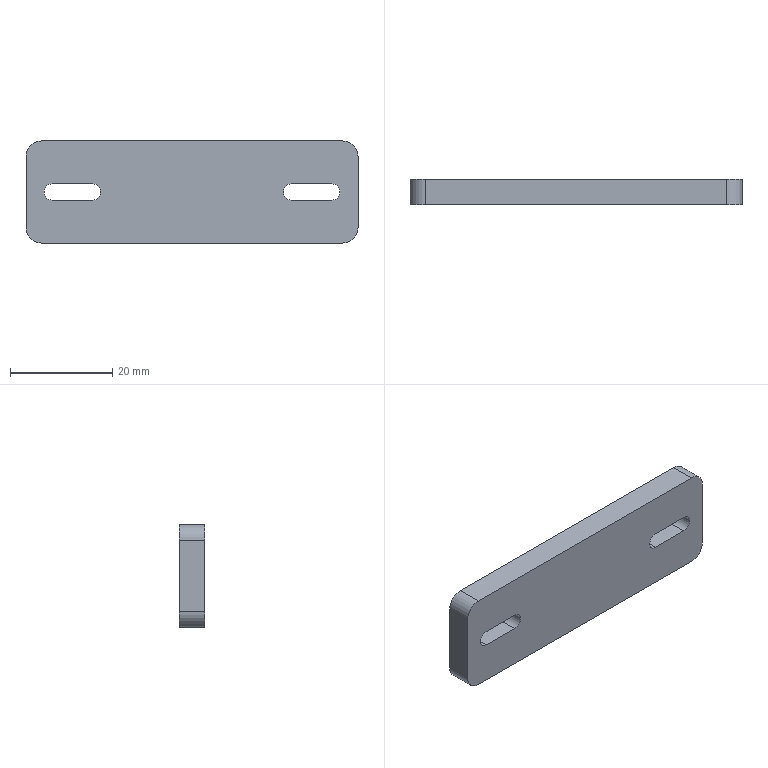Part | SolidWorks | features BaseBody 1 | 1 solid | 18 faces | box 65 x 5 x 20 mm | volume 6129 mm3 | plane 10 | cylinder 8 | commonest cylinder face diameters 3.2 x4 6 x4
STEP:
#1=CARTESIAN_POINT('',(32.5,5.,7.));
#2=VERTEX_POINT('',#1);
#3=CARTESIAN_POINT('',(32.5,5.,-7.));
#4=VERTEX_POINT('',#3);
#5=CARTESIAN_POINT('',(32.5,5.,0.));
#6=DIRECTION('',(0.,0.,-1.));
#7=VECTOR('',#6,1000.);
#8=LINE('',#5,#7);
#9=EDGE_CURVE('',#2,#4,#8,.T.);
#10=ORIENTED_EDGE('',*,*,#9,.T.);
#11=CARTESIAN_POINT('',(29.5,5.,-10.));
#12=VERTEX_POINT('',#11);
#13=CARTESIAN_POINT('',(29.5,5.,-7.));
#14=DIRECTION('',(0.,1.,0.));
#15=DIRECTION('',(0.,0.,-1.));
#16=AXIS2_PLACEMENT_3D('',#13,#14,#15);
#17=CIRCLE('',#16,3.);
#18=EDGE_CURVE('',#4,#12,#17,.T.);
#19=ORIENTED_EDGE('',*,*,#18,.T.);
#20=CARTESIAN_POINT('',(-29.5,5.,-10.));
#21=VERTEX_POINT('',#20);
#22=CARTESIAN_POINT('',(0.,5.,-10.));
#23=DIRECTION('',(-1.,0.,0.));
#24=VECTOR('',#23,1000.);
#25=LINE('',#22,#24);
#26=EDGE_CURVE('',#12,#21,#25,.T.);
#27=ORIENTED_EDGE('',*,*,#26,.T.);
#28=CARTESIAN_POINT('',(-32.5,5.,-7.));
#29=VERTEX_POINT('',#28);
#30=CARTESIAN_POINT('',(-29.5,5.,-7.));
#31=DIRECTION('',(0.,1.,0.));
#32=DIRECTION('',(0.,0.,-1.));
#33=AXIS2_PLACEMENT_3D('',#30,#31,#32);
#34=CIRCLE('',#33,3.);
#35=EDGE_CURVE('',#21,#29,#34,.T.);
#36=ORIENTED_EDGE('',*,*,#35,.T.);
#37=CARTESIAN_POINT('',(-32.5,5.,7.));
#38=VERTEX_POINT('',#37);
#39=CARTESIAN_POINT('',(-32.5,5.,0.));
#40=DIRECTION('',(0.,0.,1.));
#41=VECTOR('',#40,1000.);
#42=LINE('',#39,#41);
#43=EDGE_CURVE('',#29,#38,#42,.T.);
#44=ORIENTED_EDGE('',*,*,#43,.T.);
#45=CARTESIAN_POINT('',(-29.5,5.,10.));
#46=VERTEX_POINT('',#45);
#47=CARTESIAN_POINT('',(-29.5,5.,7.));
#48=DIRECTION('',(0.,1.,0.));
#49=DIRECTION('',(0.,0.,-1.));
#50=AXIS2_PLACEMENT_3D('',#47,#48,#49);
#51=CIRCLE('',#50,3.);
#52=EDGE_CURVE('',#38,#46,#51,.T.);
#53=ORIENTED_EDGE('',*,*,#52,.T.);
#54=CARTESIAN_POINT('',(29.5,5.,10.));
#55=VERTEX_POINT('',#54);
#56=CARTESIAN_POINT('',(0.,5.,10.));
#57=DIRECTION('',(1.,0.,0.));
#58=VECTOR('',#57,1000.);
#59=LINE('',#56,#58);
#60=EDGE_CURVE('',#46,#55,#59,.T.);
#61=ORIENTED_EDGE('',*,*,#60,.T.);
#62=CARTESIAN_POINT('',(29.5,5.,7.));
#63=DIRECTION('',(0.,1.,0.));
#64=DIRECTION('',(0.,0.,-1.));
#65=AXIS2_PLACEMENT_3D('',#62,#63,#64);
#66=CIRCLE('',#65,3.);
#67=EDGE_CURVE('',#55,#2,#66,.T.);
#68=ORIENTED_EDGE('',*,*,#67,.T.);
#69=EDGE_LOOP('',(#10,#19,#27,#36,#44,#53,#61,#68));
#70=FACE_OUTER_BOUND('',#69,.T.);
#71=CARTESIAN_POINT('',(19.5,5.,1.6));
#72=VERTEX_POINT('',#71);
#73=CARTESIAN_POINT('',(19.5,5.,-1.6));
#74=VERTEX_POINT('',#73);
#75=CARTESIAN_POINT('',(19.5,5.,0.));
#76=DIRECTION('',(0.,-1.,0.));
#77=DIRECTION('',(0.,0.,1.));
#78=AXIS2_PLACEMENT_3D('',#75,#76,#77);
#79=CIRCLE('',#78,1.6);
#80=EDGE_CURVE('',#72,#74,#79,.T.);
#81=ORIENTED_EDGE('',*,*,#80,.T.);
#82=CARTESIAN_POINT('',(27.375,5.,-1.6));
#83=VERTEX_POINT('',#82);
#84=CARTESIAN_POINT('',(0.,5.,-1.6));
#85=DIRECTION('',(1.,0.,0.));
#86=VECTOR('',#85,1000.);
#87=LINE('',#84,#86);
#88=EDGE_CURVE('',#74,#83,#87,.T.);
#89=ORIENTED_EDGE('',*,*,#88,.T.);
#90=CARTESIAN_POINT('',(27.375,5.,1.6));
#91=VERTEX_POINT('',#90);
#92=CARTESIAN_POINT('',(27.375,5.,0.));
#93=DIRECTION('',(0.,-1.,0.));
#94=DIRECTION('',(0.,0.,1.));
#95=AXIS2_PLACEMENT_3D('',#92,#93,#94);
#96=CIRCLE('',#95,1.6);
#97=EDGE_CURVE('',#83,#91,#96,.T.);
#98=ORIENTED_EDGE('',*,*,#97,.T.);
#99=CARTESIAN_POINT('',(0.,5.,1.6));
#100=DIRECTION('',(-1.,0.,0.));
#101=VECTOR('',#100,1000.);
#102=LINE('',#99,#101);
#103=EDGE_CURVE('',#91,#72,#102,.T.);
#104=ORIENTED_EDGE('',*,*,#103,.T.);
#105=EDGE_LOOP('',(#81,#89,#98,#104));
#106=FACE_BOUND('',#105,.T.);
#107=CARTESIAN_POINT('',(-19.5,5.,-1.6));
#108=VERTEX_POINT('',#107);
#109=CARTESIAN_POINT('',(-19.5,5.,1.6));
#110=VERTEX_POINT('',#109);
#111=CARTESIAN_POINT('',(-19.5,5.,0.));
#112=DIRECTION('',(0.,-1.,0.));
#113=DIRECTION('',(0.,0.,1.));
#114=AXIS2_PLACEMENT_3D('',#111,#112,#113);
#115=CIRCLE('',#114,1.6);
#116=EDGE_CURVE('',#108,#110,#115,.T.);
#117=ORIENTED_EDGE('',*,*,#116,.T.);
#118=CARTESIAN_POINT('',(-27.375,5.,1.6));
#119=VERTEX_POINT('',#118);
#120=CARTESIAN_POINT('',(0.,5.,1.6));
#121=DIRECTION('',(-1.,0.,0.));
#122=VECTOR('',#121,1000.);
#123=LINE('',#120,#122);
#124=EDGE_CURVE('',#110,#119,#123,.T.);
#125=ORIENTED_EDGE('',*,*,#124,.T.);
#126=CARTESIAN_POINT('',(-27.375,5.,-1.6));
#127=VERTEX_POINT('',#126);
#128=CARTESIAN_POINT('',(-27.375,5.,0.));
#129=DIRECTION('',(0.,-1.,0.));
#130=DIRECTION('',(0.,0.,1.));
#131=AXIS2_PLACEMENT_3D('',#128,#129,#130);
#132=CIRCLE('',#131,1.6);
#133=EDGE_CURVE('',#119,#127,#132,.T.);
#134=ORIENTED_EDGE('',*,*,#133,.T.);
#135=CARTESIAN_POINT('',(0.,5.,-1.6));
#136=DIRECTION('',(1.,0.,0.));
#137=VECTOR('',#136,1000.);
#138=LINE('',#135,#137);
#139=EDGE_CURVE('',#127,#108,#138,.T.);
#140=ORIENTED_EDGE('',*,*,#139,.T.);
#141=EDGE_LOOP('',(#117,#125,#134,#140));
#142=FACE_BOUND('',#141,.T.);
#143=CARTESIAN_POINT('',(0.,5.,0.));
#144=DIRECTION('',(0.,1.,0.));
#145=DIRECTION('',(0.,0.,1.));
#146=AXIS2_PLACEMENT_3D('',#143,#144,#145);
#147=PLANE('',#146);
#148=ADVANCED_FACE('',(#70,#106,#142),#147,.T.);
#149=CARTESIAN_POINT('',(32.5,0.,-7.));
#150=VERTEX_POINT('',#149);
#151=CARTESIAN_POINT('',(29.5,0.,-10.));
#152=VERTEX_POINT('',#151);
#153=CARTESIAN_POINT('',(29.5,0.,-7.));
#154=DIRECTION('',(0.,1.,0.));
#155=DIRECTION('',(0.,0.,-1.));
#156=AXIS2_PLACEMENT_3D('',#153,#154,#155);
#157=CIRCLE('',#156,3.);
#158=EDGE_CURVE('',#150,#152,#157,.T.);
#159=ORIENTED_EDGE('',*,*,#158,.T.);
#160=CARTESIAN_POINT('',(29.5,5.,-10.));
#161=DIRECTION('',(0.,1.,0.));
#162=VECTOR('',#161,1000.);
#163=LINE('',#160,#162);
#164=EDGE_CURVE('',#152,#12,#163,.T.);
#165=ORIENTED_EDGE('',*,*,#164,.T.);
#166=ORIENTED_EDGE('',*,*,#18,.F.);
#167=CARTESIAN_POINT('',(32.5,5.,-7.));
#168=DIRECTION('',(0.,-1.,0.));
#169=VECTOR('',#168,1000.);
#170=LINE('',#167,#169);
#171=EDGE_CURVE('',#4,#150,#170,.T.);
#172=ORIENTED_EDGE('',*,*,#171,.T.);
#173=EDGE_LOOP('',(#159,#165,#166,#172));
#174=FACE_OUTER_BOUND('',#173,.T.);
#175=CARTESIAN_POINT('',(29.5,5.,-7.));
#176=DIRECTION('',(0.,-1.,0.));
#177=DIRECTION('',(0.,0.,-1.));
#178=AXIS2_PLACEMENT_3D('',#175,#176,#177);
#179=CYLINDRICAL_SURFACE('',#178,3.);
#180=ADVANCED_FACE('',(#174),#179,.T.);
#181=ORIENTED_EDGE('',*,*,#171,.F.);
#182=ORIENTED_EDGE('',*,*,#9,.F.);
#183=CARTESIAN_POINT('',(32.5,0.,7.));
#184=VERTEX_POINT('',#183);
#185=CARTESIAN_POINT('',(32.5,5.,7.));
#186=DIRECTION('',(0.,1.,0.));
#187=VECTOR('',#186,1000.);
#188=LINE('',#185,#187);
#189=EDGE_CURVE('',#184,#2,#188,.T.);
#190=ORIENTED_EDGE('',*,*,#189,.F.);
#191=CARTESIAN_POINT('',(32.5,0.,-10.));
#192=DIRECTION('',(0.,0.,1.));
#193=VECTOR('',#192,1000.);
#194=LINE('',#191,#193);
#195=EDGE_CURVE('',#150,#184,#194,.T.);
#196=ORIENTED_EDGE('',*,*,#195,.F.);
#197=EDGE_LOOP('',(#181,#182,#190,#196));
#198=FACE_OUTER_BOUND('',#197,.T.);
#199=CARTESIAN_POINT('',(32.5,5.,-10.));
#200=DIRECTION('',(-1.,0.,0.));
#201=DIRECTION('',(0.,0.,1.));
#202=AXIS2_PLACEMENT_3D('',#199,#200,#201);
#203=PLANE('',#202);
#204=ADVANCED_FACE('',(#198),#203,.F.);
#205=CARTESIAN_POINT('',(29.5,0.,10.));
#206=VERTEX_POINT('',#205);
#207=CARTESIAN_POINT('',(29.5,0.,7.));
#208=DIRECTION('',(0.,1.,0.));
#209=DIRECTION('',(0.,0.,-1.));
#210=AXIS2_PLACEMENT_3D('',#207,#208,#209);
#211=CIRCLE('',#210,3.);
#212=EDGE_CURVE('',#206,#184,#211,.T.);
#213=ORIENTED_EDGE('',*,*,#212,.T.);
#214=ORIENTED_EDGE('',*,*,#189,.T.);
#215=ORIENTED_EDGE('',*,*,#67,.F.);
#216=CARTESIAN_POINT('',(29.5,5.,10.));
#217=DIRECTION('',(0.,-1.,0.));
#218=VECTOR('',#217,1000.);
#219=LINE('',#216,#218);
#220=EDGE_CURVE('',#55,#206,#219,.T.);
#221=ORIENTED_EDGE('',*,*,#220,.T.);
#222=EDGE_LOOP('',(#213,#214,#215,#221));
#223=FACE_OUTER_BOUND('',#222,.T.);
#224=CARTESIAN_POINT('',(29.5,5.,7.));
#225=DIRECTION('',(0.,-1.,0.));
#226=DIRECTION('',(0.,0.,-1.));
#227=AXIS2_PLACEMENT_3D('',#224,#225,#226);
#228=CYLINDRICAL_SURFACE('',#227,3.);
#229=ADVANCED_FACE('',(#223),#228,.T.);
#230=CARTESIAN_POINT('',(-29.5,0.,10.));
#231=VERTEX_POINT('',#230);
#232=CARTESIAN_POINT('',(-29.5,5.,10.));
#233=DIRECTION('',(0.,1.,0.));
#234=VECTOR('',#233,1000.);
#235=LINE('',#232,#234);
#236=EDGE_CURVE('',#231,#46,#235,.T.);
#237=ORIENTED_EDGE('',*,*,#236,.F.);
#238=CARTESIAN_POINT('',(-32.5,0.,10.));
#239=DIRECTION('',(-1.,0.,0.));
#240=VECTOR('',#239,1000.);
#241=LINE('',#238,#240);
#242=EDGE_CURVE('',#206,#231,#241,.T.);
#243=ORIENTED_EDGE('',*,*,#242,.F.);
#244=ORIENTED_EDGE('',*,*,#220,.F.);
#245=ORIENTED_EDGE('',*,*,#60,.F.);
#246=EDGE_LOOP('',(#237,#243,#244,#245));
#247=FACE_OUTER_BOUND('',#246,.T.);
#248=CARTESIAN_POINT('',(-32.5,5.,10.));
#249=DIRECTION('',(0.,0.,-1.));
#250=DIRECTION('',(-1.,0.,0.));
#251=AXIS2_PLACEMENT_3D('',#248,#249,#250);
#252=PLANE('',#251);
#253=ADVANCED_FACE('',(#247),#252,.F.);
#254=CARTESIAN_POINT('',(-32.5,0.,7.));
#255=VERTEX_POINT('',#254);
#256=CARTESIAN_POINT('',(-29.5,0.,7.));
#257=DIRECTION('',(0.,1.,0.));
#258=DIRECTION('',(0.,0.,-1.));
#259=AXIS2_PLACEMENT_3D('',#256,#257,#258);
#260=CIRCLE('',#259,3.);
#261=EDGE_CURVE('',#255,#231,#260,.T.);
#262=ORIENTED_EDGE('',*,*,#261,.T.);
#263=ORIENTED_EDGE('',*,*,#236,.T.);
#264=ORIENTED_EDGE('',*,*,#52,.F.);
#265=CARTESIAN_POINT('',(-32.5,5.,7.));
#266=DIRECTION('',(0.,-1.,0.));
#267=VECTOR('',#266,1000.);
#268=LINE('',#265,#267);
#269=EDGE_CURVE('',#38,#255,#268,.T.);
#270=ORIENTED_EDGE('',*,*,#269,.T.);
#271=EDGE_LOOP('',(#262,#263,#264,#270));
#272=FACE_OUTER_BOUND('',#271,.T.);
#273=CARTESIAN_POINT('',(-29.5,5.,7.));
#274=DIRECTION('',(0.,-1.,0.));
#275=DIRECTION('',(0.,0.,-1.));
#276=AXIS2_PLACEMENT_3D('',#273,#274,#275);
#277=CYLINDRICAL_SURFACE('',#276,3.);
#278=ADVANCED_FACE('',(#272),#277,.T.);
#279=CARTESIAN_POINT('',(-32.5,0.,-7.));
#280=VERTEX_POINT('',#279);
#281=CARTESIAN_POINT('',(-32.5,5.,-7.));
#282=DIRECTION('',(0.,1.,0.));
#283=VECTOR('',#282,1000.);
#284=LINE('',#281,#283);
#285=EDGE_CURVE('',#280,#29,#284,.T.);
#286=ORIENTED_EDGE('',*,*,#285,.F.);
#287=CARTESIAN_POINT('',(-32.5,0.,-10.));
#288=DIRECTION('',(0.,0.,-1.));
#289=VECTOR('',#288,1000.);
#290=LINE('',#287,#289);
#291=EDGE_CURVE('',#255,#280,#290,.T.);
#292=ORIENTED_EDGE('',*,*,#291,.F.);
#293=ORIENTED_EDGE('',*,*,#269,.F.);
#294=ORIENTED_EDGE('',*,*,#43,.F.);
#295=EDGE_LOOP('',(#286,#292,#293,#294));
#296=FACE_OUTER_BOUND('',#295,.T.);
#297=CARTESIAN_POINT('',(-32.5,5.,-10.));
#298=DIRECTION('',(1.,0.,0.));
#299=DIRECTION('',(0.,0.,-1.));
#300=AXIS2_PLACEMENT_3D('',#297,#298,#299);
#301=PLANE('',#300);
#302=ADVANCED_FACE('',(#296),#301,.F.);
#303=CARTESIAN_POINT('',(-29.5,0.,-10.));
#304=VERTEX_POINT('',#303);
#305=CARTESIAN_POINT('',(-29.5,0.,-7.));
#306=DIRECTION('',(0.,1.,0.));
#307=DIRECTION('',(0.,0.,-1.));
#308=AXIS2_PLACEMENT_3D('',#305,#306,#307);
#309=CIRCLE('',#308,3.);
#310=EDGE_CURVE('',#304,#280,#309,.T.);
#311=ORIENTED_EDGE('',*,*,#310,.T.);
#312=ORIENTED_EDGE('',*,*,#285,.T.);
#313=ORIENTED_EDGE('',*,*,#35,.F.);
#314=CARTESIAN_POINT('',(-29.5,5.,-10.));
#315=DIRECTION('',(0.,-1.,0.));
#316=VECTOR('',#315,1000.);
#317=LINE('',#314,#316);
#318=EDGE_CURVE('',#21,#304,#317,.T.);
#319=ORIENTED_EDGE('',*,*,#318,.T.);
#320=EDGE_LOOP('',(#311,#312,#313,#319));
#321=FACE_OUTER_BOUND('',#320,.T.);
#322=CARTESIAN_POINT('',(-29.5,5.,-7.));
#323=DIRECTION('',(0.,-1.,0.));
#324=DIRECTION('',(0.,0.,-1.));
#325=AXIS2_PLACEMENT_3D('',#322,#323,#324);
#326=CYLINDRICAL_SURFACE('',#325,3.);
#327=ADVANCED_FACE('',(#321),#326,.T.);
#328=ORIENTED_EDGE('',*,*,#318,.F.);
#329=ORIENTED_EDGE('',*,*,#26,.F.);
#330=ORIENTED_EDGE('',*,*,#164,.F.);
#331=CARTESIAN_POINT('',(-32.5,0.,-10.));
#332=DIRECTION('',(1.,0.,0.));
#333=VECTOR('',#332,1000.);
#334=LINE('',#331,#333);
#335=EDGE_CURVE('',#304,#152,#334,.T.);
#336=ORIENTED_EDGE('',*,*,#335,.F.);
#337=EDGE_LOOP('',(#328,#329,#330,#336));
#338=FACE_OUTER_BOUND('',#337,.T.);
#339=CARTESIAN_POINT('',(-32.5,5.,-10.));
#340=DIRECTION('',(0.,0.,1.));
#341=DIRECTION('',(1.,0.,0.));
#342=AXIS2_PLACEMENT_3D('',#339,#340,#341);
#343=PLANE('',#342);
#344=ADVANCED_FACE('',(#338),#343,.F.);
#345=ORIENTED_EDGE('',*,*,#88,.F.);
#346=CARTESIAN_POINT('',(19.5,0.,-1.6));
#347=VERTEX_POINT('',#346);
#348=CARTESIAN_POINT('',(19.5,-5.,-1.6));
#349=DIRECTION('',(0.,1.,0.));
#350=VECTOR('',#349,1000.);
#351=LINE('',#348,#350);
#352=EDGE_CURVE('',#347,#74,#351,.T.);
#353=ORIENTED_EDGE('',*,*,#352,.F.);
#354=CARTESIAN_POINT('',(27.375,0.,-1.6));
#355=VERTEX_POINT('',#354);
#356=CARTESIAN_POINT('',(27.375,0.,-1.6));
#357=DIRECTION('',(-1.,0.,0.));
#358=VECTOR('',#357,1000.);
#359=LINE('',#356,#358);
#360=EDGE_CURVE('',#355,#347,#359,.T.);
#361=ORIENTED_EDGE('',*,*,#360,.F.);
#362=CARTESIAN_POINT('',(27.375,-5.,-1.6));
#363=DIRECTION('',(0.,-1.,0.));
#364=VECTOR('',#363,1000.);
#365=LINE('',#362,#364);
#366=EDGE_CURVE('',#83,#355,#365,.T.);
#367=ORIENTED_EDGE('',*,*,#366,.F.);
#368=EDGE_LOOP('',(#345,#353,#361,#367));
#369=FACE_OUTER_BOUND('',#368,.T.);
#370=CARTESIAN_POINT('',(27.375,-5.,-1.6));
#371=DIRECTION('',(0.,0.,-1.));
#372=DIRECTION('',(-1.,0.,0.));
#373=AXIS2_PLACEMENT_3D('',#370,#371,#372);
#374=PLANE('',#373);
#375=ADVANCED_FACE('',(#369),#374,.F.);
#376=ORIENTED_EDGE('',*,*,#80,.F.);
#377=CARTESIAN_POINT('',(19.5,0.,1.6));
#378=VERTEX_POINT('',#377);
#379=CARTESIAN_POINT('',(19.5,-5.,1.6));
#380=DIRECTION('',(0.,1.,0.));
#381=VECTOR('',#380,1000.);
#382=LINE('',#379,#381);
#383=EDGE_CURVE('',#378,#72,#382,.T.);
#384=ORIENTED_EDGE('',*,*,#383,.F.);
#385=CARTESIAN_POINT('',(19.5,0.,0.));
#386=DIRECTION('',(0.,1.,0.));
#387=DIRECTION('',(0.,0.,1.));
#388=AXIS2_PLACEMENT_3D('',#385,#386,#387);
#389=CIRCLE('',#388,1.6);
#390=EDGE_CURVE('',#347,#378,#389,.T.);
#391=ORIENTED_EDGE('',*,*,#390,.F.);
#392=ORIENTED_EDGE('',*,*,#352,.T.);
#393=EDGE_LOOP('',(#376,#384,#391,#392));
#394=FACE_OUTER_BOUND('',#393,.T.);
#395=CARTESIAN_POINT('',(19.5,-5.,0.));
#396=DIRECTION('',(0.,1.,0.));
#397=DIRECTION('',(0.,0.,1.));
#398=AXIS2_PLACEMENT_3D('',#395,#396,#397);
#399=CYLINDRICAL_SURFACE('',#398,1.6);
#400=ADVANCED_FACE('',(#394),#399,.F.);
#401=ORIENTED_EDGE('',*,*,#103,.F.);
#402=CARTESIAN_POINT('',(27.375,0.,1.6));
#403=VERTEX_POINT('',#402);
#404=CARTESIAN_POINT('',(27.375,-5.,1.6));
#405=DIRECTION('',(0.,1.,0.));
#406=VECTOR('',#405,1000.);
#407=LINE('',#404,#406);
#408=EDGE_CURVE('',#403,#91,#407,.T.);
#409=ORIENTED_EDGE('',*,*,#408,.F.);
#410=CARTESIAN_POINT('',(27.375,0.,1.6));
#411=DIRECTION('',(1.,0.,0.));
#412=VECTOR('',#411,1000.);
#413=LINE('',#410,#412);
#414=EDGE_CURVE('',#378,#403,#413,.T.);
#415=ORIENTED_EDGE('',*,*,#414,.F.);
#416=ORIENTED_EDGE('',*,*,#383,.T.);
#417=EDGE_LOOP('',(#401,#409,#415,#416));
#418=FACE_OUTER_BOUND('',#417,.T.);
#419=CARTESIAN_POINT('',(27.375,-5.,1.6));
#420=DIRECTION('',(0.,0.,1.));
#421=DIRECTION('',(1.,0.,0.));
#422=AXIS2_PLACEMENT_3D('',#419,#420,#421);
#423=PLANE('',#422);
#424=ADVANCED_FACE('',(#418),#423,.F.);
#425=ORIENTED_EDGE('',*,*,#97,.F.);
#426=ORIENTED_EDGE('',*,*,#366,.T.);
#427=CARTESIAN_POINT('',(27.375,0.,0.));
#428=DIRECTION('',(0.,1.,0.));
#429=DIRECTION('',(0.,0.,1.));
#430=AXIS2_PLACEMENT_3D('',#427,#428,#429);
#431=CIRCLE('',#430,1.6);
#432=EDGE_CURVE('',#403,#355,#431,.T.);
#433=ORIENTED_EDGE('',*,*,#432,.F.);
#434=ORIENTED_EDGE('',*,*,#408,.T.);
#435=EDGE_LOOP('',(#425,#426,#433,#434));
#436=FACE_OUTER_BOUND('',#435,.T.);
#437=CARTESIAN_POINT('',(27.375,-5.,0.));
#438=DIRECTION('',(0.,1.,0.));
#439=DIRECTION('',(0.,0.,1.));
#440=AXIS2_PLACEMENT_3D('',#437,#438,#439);
#441=CYLINDRICAL_SURFACE('',#440,1.6);
#442=ADVANCED_FACE('',(#436),#441,.F.);
#443=ORIENTED_EDGE('',*,*,#124,.F.);
#444=CARTESIAN_POINT('',(-19.5,0.,1.6));
#445=VERTEX_POINT('',#444);
#446=CARTESIAN_POINT('',(-19.5,-5.,1.6));
#447=DIRECTION('',(0.,1.,0.));
#448=VECTOR('',#447,1000.);
#449=LINE('',#446,#448);
#450=EDGE_CURVE('',#445,#110,#449,.T.);
#451=ORIENTED_EDGE('',*,*,#450,.F.);
#452=CARTESIAN_POINT('',(-27.375,0.,1.6));
#453=VERTEX_POINT('',#452);
#454=CARTESIAN_POINT('',(-27.375,0.,1.6));
#455=DIRECTION('',(1.,0.,0.));
#456=VECTOR('',#455,1000.);
#457=LINE('',#454,#456);
#458=EDGE_CURVE('',#453,#445,#457,.T.);
#459=ORIENTED_EDGE('',*,*,#458,.F.);
#460=CARTESIAN_POINT('',(-27.375,-5.,1.6));
#461=DIRECTION('',(0.,-1.,0.));
#462=VECTOR('',#461,1000.);
#463=LINE('',#460,#462);
#464=EDGE_CURVE('',#119,#453,#463,.T.);
#465=ORIENTED_EDGE('',*,*,#464,.F.);
#466=EDGE_LOOP('',(#443,#451,#459,#465));
#467=FACE_OUTER_BOUND('',#466,.T.);
#468=CARTESIAN_POINT('',(-27.375,-5.,1.6));
#469=DIRECTION('',(0.,0.,1.));
#470=DIRECTION('',(1.,0.,0.));
#471=AXIS2_PLACEMENT_3D('',#468,#469,#470);
#472=PLANE('',#471);
#473=ADVANCED_FACE('',(#467),#472,.F.);
#474=ORIENTED_EDGE('',*,*,#116,.F.);
#475=CARTESIAN_POINT('',(-19.5,0.,-1.6));
#476=VERTEX_POINT('',#475);
#477=CARTESIAN_POINT('',(-19.5,-5.,-1.6));
#478=DIRECTION('',(0.,1.,0.));
#479=VECTOR('',#478,1000.);
#480=LINE('',#477,#479);
#481=EDGE_CURVE('',#476,#108,#480,.T.);
#482=ORIENTED_EDGE('',*,*,#481,.F.);
#483=CARTESIAN_POINT('',(-19.5,0.,0.));
#484=DIRECTION('',(0.,1.,0.));
#485=DIRECTION('',(0.,0.,1.));
#486=AXIS2_PLACEMENT_3D('',#483,#484,#485);
#487=CIRCLE('',#486,1.6);
#488=EDGE_CURVE('',#445,#476,#487,.T.);
#489=ORIENTED_EDGE('',*,*,#488,.F.);
#490=ORIENTED_EDGE('',*,*,#450,.T.);
#491=EDGE_LOOP('',(#474,#482,#489,#490));
#492=FACE_OUTER_BOUND('',#491,.T.);
#493=CARTESIAN_POINT('',(-19.5,-5.,0.));
#494=DIRECTION('',(0.,1.,0.));
#495=DIRECTION('',(0.,0.,1.));
#496=AXIS2_PLACEMENT_3D('',#493,#494,#495);
#497=CYLINDRICAL_SURFACE('',#496,1.6);
#498=ADVANCED_FACE('',(#492),#497,.F.);
#499=ORIENTED_EDGE('',*,*,#139,.F.);
#500=CARTESIAN_POINT('',(-27.375,0.,-1.6));
#501=VERTEX_POINT('',#500);
#502=CARTESIAN_POINT('',(-27.375,-5.,-1.6));
#503=DIRECTION('',(0.,1.,0.));
#504=VECTOR('',#503,1000.);
#505=LINE('',#502,#504);
#506=EDGE_CURVE('',#501,#127,#505,.T.);
#507=ORIENTED_EDGE('',*,*,#506,.F.);
#508=CARTESIAN_POINT('',(-27.375,0.,-1.6));
#509=DIRECTION('',(-1.,0.,0.));
#510=VECTOR('',#509,1000.);
#511=LINE('',#508,#510);
#512=EDGE_CURVE('',#476,#501,#511,.T.);
#513=ORIENTED_EDGE('',*,*,#512,.F.);
#514=ORIENTED_EDGE('',*,*,#481,.T.);
#515=EDGE_LOOP('',(#499,#507,#513,#514));
#516=FACE_OUTER_BOUND('',#515,.T.);
#517=CARTESIAN_POINT('',(-27.375,-5.,-1.6));
#518=DIRECTION('',(0.,0.,-1.));
#519=DIRECTION('',(-1.,0.,0.));
#520=AXIS2_PLACEMENT_3D('',#517,#518,#519);
#521=PLANE('',#520);
#522=ADVANCED_FACE('',(#516),#521,.F.);
#523=ORIENTED_EDGE('',*,*,#133,.F.);
#524=ORIENTED_EDGE('',*,*,#464,.T.);
#525=CARTESIAN_POINT('',(-27.375,0.,0.));
#526=DIRECTION('',(0.,1.,0.));
#527=DIRECTION('',(0.,0.,1.));
#528=AXIS2_PLACEMENT_3D('',#525,#526,#527);
#529=CIRCLE('',#528,1.6);
#530=EDGE_CURVE('',#501,#453,#529,.T.);
#531=ORIENTED_EDGE('',*,*,#530,.F.);
#532=ORIENTED_EDGE('',*,*,#506,.T.);
#533=EDGE_LOOP('',(#523,#524,#531,#532));
#534=FACE_OUTER_BOUND('',#533,.T.);
#535=CARTESIAN_POINT('',(-27.375,-5.,0.));
#536=DIRECTION('',(0.,1.,0.));
#537=DIRECTION('',(0.,0.,1.));
#538=AXIS2_PLACEMENT_3D('',#535,#536,#537);
#539=CYLINDRICAL_SURFACE('',#538,1.6);
#540=ADVANCED_FACE('',(#534),#539,.F.);
#541=ORIENTED_EDGE('',*,*,#310,.F.);
#542=ORIENTED_EDGE('',*,*,#335,.T.);
#543=ORIENTED_EDGE('',*,*,#158,.F.);
#544=ORIENTED_EDGE('',*,*,#195,.T.);
#545=ORIENTED_EDGE('',*,*,#212,.F.);
#546=ORIENTED_EDGE('',*,*,#242,.T.);
#547=ORIENTED_EDGE('',*,*,#261,.F.);
#548=ORIENTED_EDGE('',*,*,#291,.T.);
#549=EDGE_LOOP('',(#541,#542,#543,#544,#545,#546,#547,#548));
#550=FACE_OUTER_BOUND('',#549,.T.);
#551=ORIENTED_EDGE('',*,*,#432,.T.);
#552=ORIENTED_EDGE('',*,*,#360,.T.);
#553=ORIENTED_EDGE('',*,*,#390,.T.);
#554=ORIENTED_EDGE('',*,*,#414,.T.);
#555=EDGE_LOOP('',(#551,#552,#553,#554));
#556=FACE_BOUND('',#555,.T.);
#557=ORIENTED_EDGE('',*,*,#530,.T.);
#558=ORIENTED_EDGE('',*,*,#458,.T.);
#559=ORIENTED_EDGE('',*,*,#488,.T.);
#560=ORIENTED_EDGE('',*,*,#512,.T.);
#561=EDGE_LOOP('',(#557,#558,#559,#560));
#562=FACE_BOUND('',#561,.T.);
#563=CARTESIAN_POINT('',(0.,0.,0.));
#564=DIRECTION('',(0.,1.,0.));
#565=DIRECTION('',(0.,0.,1.));
#566=AXIS2_PLACEMENT_3D('',#563,#564,#565);
#567=PLANE('',#566);
#568=ADVANCED_FACE('',(#550,#556,#562),#567,.F.);
#569=CLOSED_SHELL('',(#148,#180,#204,#229,#253,#278,#302,#327,#344,#375,#400,#424,#442,#473,#498,#522,#540,#568));
#570=MANIFOLD_SOLID_BREP('',#569);
#571=CARTESIAN_POINT('',(0.,0.,0.));
#572=DIRECTION('',(0.,0.,1.));
#573=DIRECTION('',(1.,0.,0.));
#574=AXIS2_PLACEMENT_3D('',#571,#572,#573);
#575=(LENGTH_UNIT()NAMED_UNIT(*)SI_UNIT(.MILLI.,.METRE.));
#576=UNCERTAINTY_MEASURE_WITH_UNIT(LENGTH_MEASURE(0.00001),#575,'','');
#577=(NAMED_UNIT(*)PLANE_ANGLE_UNIT()SI_UNIT($,.RADIAN.));
#578=(NAMED_UNIT(*)SI_UNIT($,.STERADIAN.)SOLID_ANGLE_UNIT());
#579=(GEOMETRIC_REPRESENTATION_CONTEXT(3)GLOBAL_UNCERTAINTY_ASSIGNED_CONTEXT((#576))GLOBAL_UNIT_ASSIGNED_CONTEXT((#575,#577,#578))REPRESENTATION_CONTEXT('',''));
#580=ADVANCED_BREP_SHAPE_REPRESENTATION('',(#570,#574),#579);